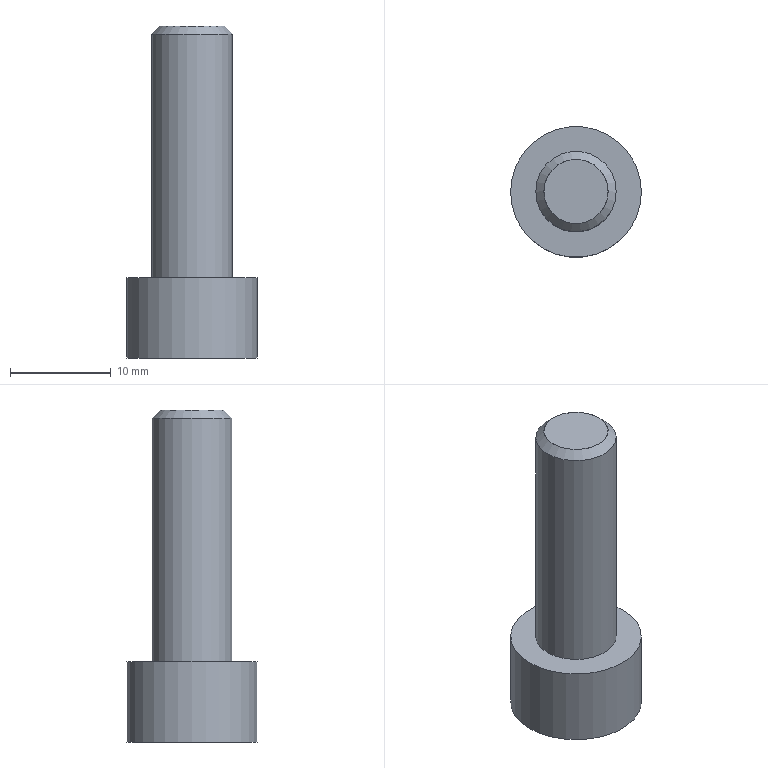Part | STEP file | lll_id2566_x_t | 1 solid | 16 faces | box 13 x 13 x 33 mm | volume 2183 mm3 | plane 11 | cylinder 4 | cone 1 | commonest cylinder face diameters 6.38 x1 6.4 x1 8 x1 13 x1
STEP:
#1=CARTESIAN_POINT('',(456.435,-449.,61.9));
#2=VERTEX_POINT('',#1);
#3=CARTESIAN_POINT('',(452.435,-449.,61.9));
#4=DIRECTION('',(0.,0.,-1.));
#5=DIRECTION('',(1.,0.,0.));
#6=AXIS2_PLACEMENT_3D('',#3,#4,#5);
#7=CIRCLE('',#6,4.);
#8=EDGE_CURVE('',#2,#2,#7,.T.);
#9=ORIENTED_EDGE('',*,*,#8,.T.);
#10=EDGE_LOOP('',(#9));
#11=FACE_BOUND('',#10,.T.);
#12=CARTESIAN_POINT('',(445.935,-449.,61.9));
#13=VERTEX_POINT('',#12);
#14=CARTESIAN_POINT('',(452.435,-449.,61.9));
#15=DIRECTION('',(0.,0.,1.));
#16=DIRECTION('',(-1.,0.,0.));
#17=AXIS2_PLACEMENT_3D('',#14,#15,#16);
#18=CIRCLE('',#17,6.5);
#19=EDGE_CURVE('',#13,#13,#18,.T.);
#20=ORIENTED_EDGE('',*,*,#19,.T.);
#21=EDGE_LOOP('',(#20));
#22=FACE_BOUND('',#21,.T.);
#23=CARTESIAN_POINT('',(452.435,-449.,61.9));
#24=DIRECTION('',(0.,0.,1.));
#25=DIRECTION('',(1.,0.,0.));
#26=AXIS2_PLACEMENT_3D('',#23,#24,#25);
#27=PLANE('',#26);
#28=ADVANCED_FACE('',(#11,#22),#27,.T.);
#29=CARTESIAN_POINT('',(452.435,-452.47,53.9));
#30=VERTEX_POINT('',#29);
#31=CARTESIAN_POINT('',(455.435,-450.738,53.9));
#32=VERTEX_POINT('',#31);
#33=CARTESIAN_POINT('',(453.936,-451.604,53.9));
#34=DIRECTION('',(0.866,0.5,0.));
#35=VECTOR('',#34,1.);
#36=LINE('',#33,#35);
#37=EDGE_CURVE('',#30,#32,#36,.T.);
#38=ORIENTED_EDGE('',*,*,#37,.T.);
#39=CARTESIAN_POINT('',(455.435,-447.272,53.9));
#40=VERTEX_POINT('',#39);
#41=CARTESIAN_POINT('',(455.435,-449.005,53.9));
#42=DIRECTION('',(0.,-1.,0.));
#43=VECTOR('',#42,1.);
#44=LINE('',#41,#43);
#45=EDGE_CURVE('',#40,#32,#44,.T.);
#46=ORIENTED_EDGE('',*,*,#45,.F.);
#47=CARTESIAN_POINT('',(452.435,-445.54,53.9));
#48=VERTEX_POINT('',#47);
#49=CARTESIAN_POINT('',(453.936,-446.406,53.9));
#50=DIRECTION('',(-0.866,0.5,0.));
#51=VECTOR('',#50,1.);
#52=LINE('',#49,#51);
#53=EDGE_CURVE('',#40,#48,#52,.T.);
#54=ORIENTED_EDGE('',*,*,#53,.T.);
#55=CARTESIAN_POINT('',(449.435,-447.272,53.9));
#56=VERTEX_POINT('',#55);
#57=CARTESIAN_POINT('',(450.935,-446.406,53.9));
#58=DIRECTION('',(-0.866,-0.5,0.));
#59=VECTOR('',#58,1.);
#60=LINE('',#57,#59);
#61=EDGE_CURVE('',#48,#56,#60,.T.);
#62=ORIENTED_EDGE('',*,*,#61,.T.);
#63=CARTESIAN_POINT('',(449.435,-450.738,53.9));
#64=VERTEX_POINT('',#63);
#65=CARTESIAN_POINT('',(449.435,-449.005,53.9));
#66=DIRECTION('',(0.,1.,0.));
#67=VECTOR('',#66,1.);
#68=LINE('',#65,#67);
#69=EDGE_CURVE('',#64,#56,#68,.T.);
#70=ORIENTED_EDGE('',*,*,#69,.F.);
#71=CARTESIAN_POINT('',(450.935,-451.604,53.9));
#72=DIRECTION('',(0.866,-0.5,0.));
#73=VECTOR('',#72,1.);
#74=LINE('',#71,#73);
#75=EDGE_CURVE('',#64,#30,#74,.T.);
#76=ORIENTED_EDGE('',*,*,#75,.T.);
#77=EDGE_LOOP('',(#38,#46,#54,#62,#70,#76));
#78=FACE_BOUND('',#77,.T.);
#79=CARTESIAN_POINT('',(445.935,-449.,53.9));
#80=VERTEX_POINT('',#79);
#81=CARTESIAN_POINT('',(452.435,-449.,53.9));
#82=DIRECTION('',(0.,0.,-1.));
#83=DIRECTION('',(-1.,0.,0.));
#84=AXIS2_PLACEMENT_3D('',#81,#82,#83);
#85=CIRCLE('',#84,6.5);
#86=EDGE_CURVE('',#80,#80,#85,.T.);
#87=ORIENTED_EDGE('',*,*,#86,.T.);
#88=EDGE_LOOP('',(#87));
#89=FACE_BOUND('',#88,.T.);
#90=CARTESIAN_POINT('',(452.435,-449.,53.9));
#91=DIRECTION('',(0.,0.,-1.));
#92=DIRECTION('',(-1.,0.,0.));
#93=AXIS2_PLACEMENT_3D('',#90,#91,#92);
#94=PLANE('',#93);
#95=ADVANCED_FACE('',(#78,#89),#94,.T.);
#96=ORIENTED_EDGE('',*,*,#19,.F.);
#97=EDGE_LOOP('',(#96));
#98=FACE_BOUND('',#97,.T.);
#99=ORIENTED_EDGE('',*,*,#86,.F.);
#100=EDGE_LOOP('',(#99));
#101=FACE_BOUND('',#100,.T.);
#102=CARTESIAN_POINT('',(452.435,-449.,52.9));
#103=DIRECTION('',(0.,0.,1.));
#104=DIRECTION('',(1.,0.,0.));
#105=AXIS2_PLACEMENT_3D('',#102,#103,#104);
#106=CYLINDRICAL_SURFACE('',#105,6.5);
#107=ADVANCED_FACE('',(#98,#101),#106,.T.);
#108=CARTESIAN_POINT('',(448.435,-449.,86.1));
#109=VERTEX_POINT('',#108);
#110=CARTESIAN_POINT('',(452.435,-449.,86.1));
#111=DIRECTION('',(0.,0.,1.));
#112=DIRECTION('',(-1.,0.,0.));
#113=AXIS2_PLACEMENT_3D('',#110,#111,#112);
#114=CIRCLE('',#113,4.);
#115=EDGE_CURVE('',#109,#109,#114,.T.);
#116=ORIENTED_EDGE('',*,*,#115,.F.);
#117=EDGE_LOOP('',(#116));
#118=FACE_BOUND('',#117,.T.);
#119=ORIENTED_EDGE('',*,*,#8,.F.);
#120=EDGE_LOOP('',(#119));
#121=FACE_BOUND('',#120,.T.);
#122=CARTESIAN_POINT('',(452.435,-449.,52.9));
#123=DIRECTION('',(0.,0.,1.));
#124=DIRECTION('',(1.,0.,0.));
#125=AXIS2_PLACEMENT_3D('',#122,#123,#124);
#126=CYLINDRICAL_SURFACE('',#125,4.);
#127=ADVANCED_FACE('',(#118,#121),#126,.T.);
#128=CARTESIAN_POINT('',(455.435,-450.738,57.9));
#129=VERTEX_POINT('',#128);
#130=CARTESIAN_POINT('',(455.435,-447.272,57.9));
#131=VERTEX_POINT('',#130);
#132=CARTESIAN_POINT('',(455.435,-449.005,57.9));
#133=DIRECTION('',(0.,1.,0.));
#134=VECTOR('',#133,1.);
#135=LINE('',#132,#134);
#136=EDGE_CURVE('',#129,#131,#135,.T.);
#137=ORIENTED_EDGE('',*,*,#136,.T.);
#138=CARTESIAN_POINT('',(455.435,-447.272,57.9));
#139=DIRECTION('',(0.,0.,-1.));
#140=VECTOR('',#139,1.);
#141=LINE('',#138,#140);
#142=EDGE_CURVE('',#131,#40,#141,.T.);
#143=ORIENTED_EDGE('',*,*,#142,.T.);
#144=ORIENTED_EDGE('',*,*,#45,.T.);
#145=CARTESIAN_POINT('',(455.435,-450.738,57.9));
#146=DIRECTION('',(0.,0.,1.));
#147=VECTOR('',#146,1.);
#148=LINE('',#145,#147);
#149=EDGE_CURVE('',#32,#129,#148,.T.);
#150=ORIENTED_EDGE('',*,*,#149,.T.);
#151=EDGE_LOOP('',(#137,#143,#144,#150));
#152=FACE_OUTER_BOUND('',#151,.T.);
#153=CARTESIAN_POINT('',(455.435,-449.005,57.9));
#154=DIRECTION('',(1.,0.,0.));
#155=DIRECTION('',(0.,0.,-1.));
#156=AXIS2_PLACEMENT_3D('',#153,#154,#155);
#157=PLANE('',#156);
#158=ADVANCED_FACE('',(#152),#157,.F.);
#159=CARTESIAN_POINT('',(449.435,-447.272,57.9));
#160=VERTEX_POINT('',#159);
#161=CARTESIAN_POINT('',(452.435,-445.54,57.9));
#162=VERTEX_POINT('',#161);
#163=CARTESIAN_POINT('',(450.935,-446.406,57.9));
#164=DIRECTION('',(0.866,0.5,0.));
#165=VECTOR('',#164,1.);
#166=LINE('',#163,#165);
#167=EDGE_CURVE('',#160,#162,#166,.T.);
#168=ORIENTED_EDGE('',*,*,#167,.T.);
#169=CARTESIAN_POINT('',(453.936,-446.406,57.9));
#170=DIRECTION('',(0.866,-0.5,0.));
#171=VECTOR('',#170,1.);
#172=LINE('',#169,#171);
#173=EDGE_CURVE('',#162,#131,#172,.T.);
#174=ORIENTED_EDGE('',*,*,#173,.T.);
#175=ORIENTED_EDGE('',*,*,#136,.F.);
#176=CARTESIAN_POINT('',(452.435,-452.47,57.9));
#177=VERTEX_POINT('',#176);
#178=CARTESIAN_POINT('',(453.936,-451.604,57.9));
#179=DIRECTION('',(-0.866,-0.5,0.));
#180=VECTOR('',#179,1.);
#181=LINE('',#178,#180);
#182=EDGE_CURVE('',#129,#177,#181,.T.);
#183=ORIENTED_EDGE('',*,*,#182,.T.);
#184=CARTESIAN_POINT('',(449.435,-450.738,57.9));
#185=VERTEX_POINT('',#184);
#186=CARTESIAN_POINT('',(450.935,-451.604,57.9));
#187=DIRECTION('',(-0.866,0.5,0.));
#188=VECTOR('',#187,1.);
#189=LINE('',#186,#188);
#190=EDGE_CURVE('',#177,#185,#189,.T.);
#191=ORIENTED_EDGE('',*,*,#190,.T.);
#192=CARTESIAN_POINT('',(449.435,-449.005,57.9));
#193=DIRECTION('',(0.,-1.,0.));
#194=VECTOR('',#193,1.);
#195=LINE('',#192,#194);
#196=EDGE_CURVE('',#160,#185,#195,.T.);
#197=ORIENTED_EDGE('',*,*,#196,.F.);
#198=EDGE_LOOP('',(#168,#174,#175,#183,#191,#197));
#199=FACE_OUTER_BOUND('',#198,.T.);
#200=CARTESIAN_POINT('',(452.435,-449.005,57.9));
#201=DIRECTION('',(0.,0.,1.));
#202=DIRECTION('',(1.,0.,0.));
#203=AXIS2_PLACEMENT_3D('',#200,#201,#202);
#204=PLANE('',#203);
#205=ADVANCED_FACE('',(#199),#204,.F.);
#206=ORIENTED_EDGE('',*,*,#69,.T.);
#207=CARTESIAN_POINT('',(449.435,-447.272,57.9));
#208=DIRECTION('',(0.,0.,1.));
#209=VECTOR('',#208,1.);
#210=LINE('',#207,#209);
#211=EDGE_CURVE('',#56,#160,#210,.T.);
#212=ORIENTED_EDGE('',*,*,#211,.T.);
#213=ORIENTED_EDGE('',*,*,#196,.T.);
#214=CARTESIAN_POINT('',(449.435,-450.738,57.9));
#215=DIRECTION('',(0.,0.,-1.));
#216=VECTOR('',#215,1.);
#217=LINE('',#214,#216);
#218=EDGE_CURVE('',#185,#64,#217,.T.);
#219=ORIENTED_EDGE('',*,*,#218,.T.);
#220=EDGE_LOOP('',(#206,#212,#213,#219));
#221=FACE_OUTER_BOUND('',#220,.T.);
#222=CARTESIAN_POINT('',(449.435,-449.005,57.9));
#223=DIRECTION('',(-1.,0.,0.));
#224=DIRECTION('',(0.,0.,1.));
#225=AXIS2_PLACEMENT_3D('',#222,#223,#224);
#226=PLANE('',#225);
#227=ADVANCED_FACE('',(#221),#226,.F.);
#228=ORIENTED_EDGE('',*,*,#182,.F.);
#229=ORIENTED_EDGE('',*,*,#149,.F.);
#230=ORIENTED_EDGE('',*,*,#37,.F.);
#231=CARTESIAN_POINT('',(452.435,-452.47,57.9));
#232=DIRECTION('',(0.,0.,-1.));
#233=VECTOR('',#232,1.);
#234=LINE('',#231,#233);
#235=EDGE_CURVE('',#177,#30,#234,.T.);
#236=ORIENTED_EDGE('',*,*,#235,.F.);
#237=EDGE_LOOP('',(#228,#229,#230,#236));
#238=FACE_OUTER_BOUND('',#237,.T.);
#239=CARTESIAN_POINT('',(452.435,-452.47,57.9));
#240=DIRECTION('',(-0.5,0.866,0.));
#241=DIRECTION('',(-0.866,-0.5,0.));
#242=AXIS2_PLACEMENT_3D('',#239,#240,#241);
#243=PLANE('',#242);
#244=ADVANCED_FACE('',(#238),#243,.T.);
#245=ORIENTED_EDGE('',*,*,#190,.F.);
#246=ORIENTED_EDGE('',*,*,#235,.T.);
#247=ORIENTED_EDGE('',*,*,#75,.F.);
#248=ORIENTED_EDGE('',*,*,#218,.F.);
#249=EDGE_LOOP('',(#245,#246,#247,#248));
#250=FACE_OUTER_BOUND('',#249,.T.);
#251=CARTESIAN_POINT('',(449.435,-450.738,57.9));
#252=DIRECTION('',(0.5,0.866,0.));
#253=DIRECTION('',(-0.866,0.5,0.));
#254=AXIS2_PLACEMENT_3D('',#251,#252,#253);
#255=PLANE('',#254);
#256=ADVANCED_FACE('',(#250),#255,.T.);
#257=ORIENTED_EDGE('',*,*,#167,.F.);
#258=ORIENTED_EDGE('',*,*,#211,.F.);
#259=ORIENTED_EDGE('',*,*,#61,.F.);
#260=CARTESIAN_POINT('',(452.435,-445.54,57.9));
#261=DIRECTION('',(0.,0.,-1.));
#262=VECTOR('',#261,1.);
#263=LINE('',#260,#262);
#264=EDGE_CURVE('',#162,#48,#263,.T.);
#265=ORIENTED_EDGE('',*,*,#264,.F.);
#266=EDGE_LOOP('',(#257,#258,#259,#265));
#267=FACE_OUTER_BOUND('',#266,.T.);
#268=CARTESIAN_POINT('',(452.435,-445.54,57.9));
#269=DIRECTION('',(0.5,-0.866,0.));
#270=DIRECTION('',(0.866,0.5,0.));
#271=AXIS2_PLACEMENT_3D('',#268,#269,#270);
#272=PLANE('',#271);
#273=ADVANCED_FACE('',(#267),#272,.T.);
#274=ORIENTED_EDGE('',*,*,#173,.F.);
#275=ORIENTED_EDGE('',*,*,#264,.T.);
#276=ORIENTED_EDGE('',*,*,#53,.F.);
#277=ORIENTED_EDGE('',*,*,#142,.F.);
#278=EDGE_LOOP('',(#274,#275,#276,#277));
#279=FACE_OUTER_BOUND('',#278,.T.);
#280=CARTESIAN_POINT('',(455.435,-447.272,57.9));
#281=DIRECTION('',(-0.5,-0.866,0.));
#282=DIRECTION('',(0.866,-0.5,0.));
#283=AXIS2_PLACEMENT_3D('',#280,#281,#282);
#284=PLANE('',#283);
#285=ADVANCED_FACE('',(#279),#284,.T.);
#286=CARTESIAN_POINT('',(449.235,-449.,86.9));
#287=VERTEX_POINT('',#286);
#288=CARTESIAN_POINT('',(452.435,-449.,86.9));
#289=DIRECTION('',(0.,0.,-1.));
#290=DIRECTION('',(-1.,0.,0.));
#291=AXIS2_PLACEMENT_3D('',#288,#289,#290);
#292=CIRCLE('',#291,3.2);
#293=EDGE_CURVE('',#287,#287,#292,.T.);
#294=ORIENTED_EDGE('',*,*,#293,.T.);
#295=EDGE_LOOP('',(#294));
#296=FACE_BOUND('',#295,.T.);
#297=ORIENTED_EDGE('',*,*,#115,.T.);
#298=EDGE_LOOP('',(#297));
#299=FACE_BOUND('',#298,.T.);
#300=CARTESIAN_POINT('',(452.435,-449.,86.1));
#301=DIRECTION('',(0.,0.,-1.));
#302=DIRECTION('',(-1.,0.,0.));
#303=AXIS2_PLACEMENT_3D('',#300,#301,#302);
#304=CONICAL_SURFACE('',#303,4.,45.);
#305=ADVANCED_FACE('',(#296,#299),#304,.T.);
#306=CARTESIAN_POINT('',(449.245,-449.,70.9));
#307=VERTEX_POINT('',#306);
#308=CARTESIAN_POINT('',(452.435,-449.,70.9));
#309=DIRECTION('',(0.,0.,-1.));
#310=DIRECTION('',(-1.,0.,0.));
#311=AXIS2_PLACEMENT_3D('',#308,#309,#310);
#312=CIRCLE('',#311,3.19);
#313=EDGE_CURVE('',#307,#307,#312,.T.);
#314=ORIENTED_EDGE('',*,*,#313,.T.);
#315=EDGE_LOOP('',(#314));
#316=FACE_BOUND('',#315,.T.);
#317=CARTESIAN_POINT('',(455.635,-449.,70.9));
#318=VERTEX_POINT('',#317);
#319=CARTESIAN_POINT('',(452.435,-449.,70.9));
#320=DIRECTION('',(0.,0.,-1.));
#321=DIRECTION('',(1.,0.,0.));
#322=AXIS2_PLACEMENT_3D('',#319,#320,#321);
#323=CIRCLE('',#322,3.2);
#324=EDGE_CURVE('',#318,#318,#323,.T.);
#325=ORIENTED_EDGE('',*,*,#324,.F.);
#326=EDGE_LOOP('',(#325));
#327=FACE_BOUND('',#326,.T.);
#328=CARTESIAN_POINT('',(452.435,-449.,70.9));
#329=DIRECTION('',(0.,0.,-1.));
#330=DIRECTION('',(-1.,0.,0.));
#331=AXIS2_PLACEMENT_3D('',#328,#329,#330);
#332=PLANE('',#331);
#333=ADVANCED_FACE('',(#316,#327),#332,.F.);
#334=ORIENTED_EDGE('',*,*,#313,.F.);
#335=EDGE_LOOP('',(#334));
#336=FACE_BOUND('',#335,.T.);
#337=CARTESIAN_POINT('',(455.625,-449.,86.9));
#338=VERTEX_POINT('',#337);
#339=CARTESIAN_POINT('',(452.435,-449.,86.9));
#340=DIRECTION('',(0.,0.,-1.));
#341=DIRECTION('',(1.,0.,0.));
#342=AXIS2_PLACEMENT_3D('',#339,#340,#341);
#343=CIRCLE('',#342,3.19);
#344=EDGE_CURVE('',#338,#338,#343,.T.);
#345=ORIENTED_EDGE('',*,*,#344,.T.);
#346=EDGE_LOOP('',(#345));
#347=FACE_BOUND('',#346,.T.);
#348=CARTESIAN_POINT('',(452.435,-449.,86.9));
#349=DIRECTION('',(0.,0.,-1.));
#350=DIRECTION('',(-1.,0.,0.));
#351=AXIS2_PLACEMENT_3D('',#348,#349,#350);
#352=CYLINDRICAL_SURFACE('',#351,3.19);
#353=ADVANCED_FACE('',(#336,#347),#352,.T.);
#354=ORIENTED_EDGE('',*,*,#324,.T.);
#355=EDGE_LOOP('',(#354));
#356=FACE_BOUND('',#355,.T.);
#357=ORIENTED_EDGE('',*,*,#293,.F.);
#358=EDGE_LOOP('',(#357));
#359=FACE_BOUND('',#358,.T.);
#360=CARTESIAN_POINT('',(452.435,-449.,86.9));
#361=DIRECTION('',(0.,0.,-1.));
#362=DIRECTION('',(-1.,0.,0.));
#363=AXIS2_PLACEMENT_3D('',#360,#361,#362);
#364=CYLINDRICAL_SURFACE('',#363,3.2);
#365=ADVANCED_FACE('',(#356,#359),#364,.F.);
#366=ORIENTED_EDGE('',*,*,#344,.F.);
#367=EDGE_LOOP('',(#366));
#368=FACE_OUTER_BOUND('',#367,.T.);
#369=CARTESIAN_POINT('',(452.435,-449.,86.9));
#370=DIRECTION('',(0.,0.,1.));
#371=DIRECTION('',(1.,0.,0.));
#372=AXIS2_PLACEMENT_3D('',#369,#370,#371);
#373=PLANE('',#372);
#374=ADVANCED_FACE('',(#368),#373,.T.);
#375=CLOSED_SHELL('',(#28,#95,#107,#127,#158,#205,#227,#244,#256,#273,#285,#305,#333,#353,#365,#374));
#376=MANIFOLD_SOLID_BREP('',#375);
#377=(LENGTH_UNIT()NAMED_UNIT(*)SI_UNIT(.MILLI.,.METRE.));
#378=UNCERTAINTY_MEASURE_WITH_UNIT(LENGTH_MEASURE(0.00002),#377,'','');
#379=(NAMED_UNIT(*)PLANE_ANGLE_UNIT()SI_UNIT($,.RADIAN.));
#380=PLANE_ANGLE_MEASURE_WITH_UNIT(PLANE_ANGLE_MEASURE(0.01745),#379);
#381=DIMENSIONAL_EXPONENTS(0.,0.,0.,0.,0.,0.,0.);
#382=(CONVERSION_BASED_UNIT('DEGREE',#380)NAMED_UNIT(#381)PLANE_ANGLE_UNIT());
#383=(NAMED_UNIT(*)SI_UNIT($,.STERADIAN.)SOLID_ANGLE_UNIT());
#384=(GEOMETRIC_REPRESENTATION_CONTEXT(3)GLOBAL_UNCERTAINTY_ASSIGNED_CONTEXT((#378))GLOBAL_UNIT_ASSIGNED_CONTEXT((#377,#382,#383))REPRESENTATION_CONTEXT('',''));
#385=ADVANCED_BREP_SHAPE_REPRESENTATION('',(#376),#384);